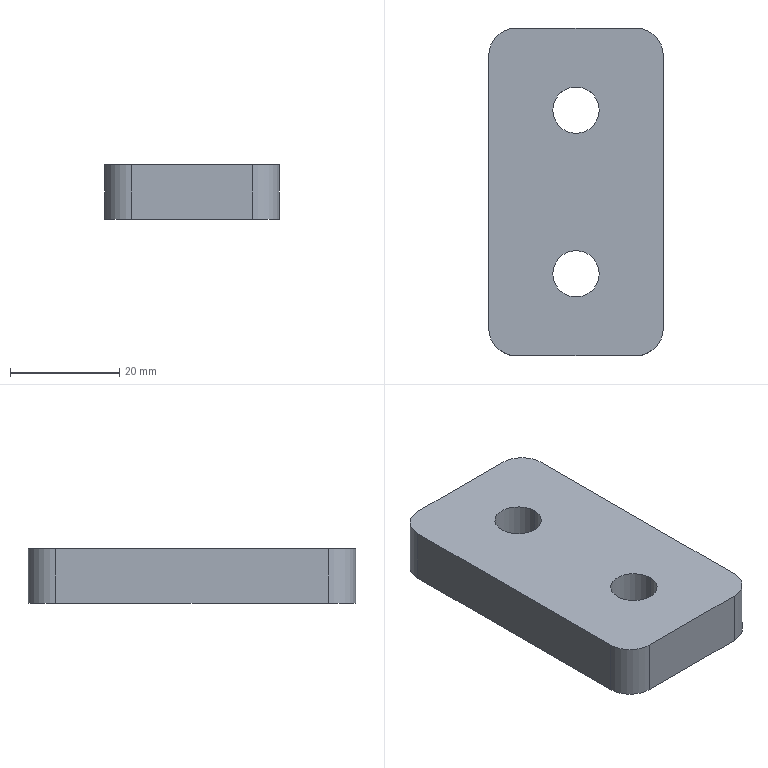Part | SolidWorks | features BaseBody 1 | 1 solid | 14 faces | box 32 x 60 x 10 mm | volume 17850 mm3 | cylinder 8 | plane 6 | commonest cylinder face diameters 8.5 x4 10 x4
STEP:
#1=CARTESIAN_POINT('',(-4.25,15.,0.));
#2=VERTEX_POINT('',#1);
#3=CARTESIAN_POINT('',(-4.25,15.,10.));
#4=VERTEX_POINT('',#3);
#5=CARTESIAN_POINT('',(-4.25,15.,-10.));
#6=DIRECTION('',(0.,0.,1.));
#7=VECTOR('',#6,1000.);
#8=LINE('',#5,#7);
#9=EDGE_CURVE('',#2,#4,#8,.T.);
#10=ORIENTED_EDGE('',*,*,#9,.F.);
#11=CARTESIAN_POINT('',(4.25,15.,0.));
#12=VERTEX_POINT('',#11);
#13=CARTESIAN_POINT('',(0.,15.,0.));
#14=DIRECTION('',(0.,0.,1.));
#15=DIRECTION('',(1.,0.,0.));
#16=AXIS2_PLACEMENT_3D('',#13,#14,#15);
#17=CIRCLE('',#16,4.25);
#18=EDGE_CURVE('',#12,#2,#17,.T.);
#19=ORIENTED_EDGE('',*,*,#18,.F.);
#20=CARTESIAN_POINT('',(4.25,15.,10.));
#21=VERTEX_POINT('',#20);
#22=CARTESIAN_POINT('',(4.25,15.,-10.));
#23=DIRECTION('',(0.,0.,1.));
#24=VECTOR('',#23,1000.);
#25=LINE('',#22,#24);
#26=EDGE_CURVE('',#12,#21,#25,.T.);
#27=ORIENTED_EDGE('',*,*,#26,.T.);
#28=CARTESIAN_POINT('',(0.,15.,10.));
#29=DIRECTION('',(0.,0.,1.));
#30=DIRECTION('',(1.,0.,0.));
#31=AXIS2_PLACEMENT_3D('',#28,#29,#30);
#32=CIRCLE('',#31,4.25);
#33=EDGE_CURVE('',#21,#4,#32,.T.);
#34=ORIENTED_EDGE('',*,*,#33,.T.);
#35=EDGE_LOOP('',(#10,#19,#27,#34));
#36=FACE_OUTER_BOUND('',#35,.T.);
#37=CARTESIAN_POINT('',(0.,15.,-10.));
#38=DIRECTION('',(0.,0.,1.));
#39=DIRECTION('',(1.,0.,0.));
#40=AXIS2_PLACEMENT_3D('',#37,#38,#39);
#41=CYLINDRICAL_SURFACE('',#40,4.25);
#42=ADVANCED_FACE('',(#36),#41,.F.);
#43=CARTESIAN_POINT('',(-4.25,-15.,0.));
#44=VERTEX_POINT('',#43);
#45=CARTESIAN_POINT('',(-4.25,-15.,10.));
#46=VERTEX_POINT('',#45);
#47=CARTESIAN_POINT('',(-4.25,-15.,-10.));
#48=DIRECTION('',(0.,0.,1.));
#49=VECTOR('',#48,1000.);
#50=LINE('',#47,#49);
#51=EDGE_CURVE('',#44,#46,#50,.T.);
#52=ORIENTED_EDGE('',*,*,#51,.F.);
#53=CARTESIAN_POINT('',(4.25,-15.,0.));
#54=VERTEX_POINT('',#53);
#55=CARTESIAN_POINT('',(0.,-15.,0.));
#56=DIRECTION('',(0.,0.,1.));
#57=DIRECTION('',(1.,0.,0.));
#58=AXIS2_PLACEMENT_3D('',#55,#56,#57);
#59=CIRCLE('',#58,4.25);
#60=EDGE_CURVE('',#54,#44,#59,.T.);
#61=ORIENTED_EDGE('',*,*,#60,.F.);
#62=CARTESIAN_POINT('',(4.25,-15.,10.));
#63=VERTEX_POINT('',#62);
#64=CARTESIAN_POINT('',(4.25,-15.,-10.));
#65=DIRECTION('',(0.,0.,1.));
#66=VECTOR('',#65,1000.);
#67=LINE('',#64,#66);
#68=EDGE_CURVE('',#54,#63,#67,.T.);
#69=ORIENTED_EDGE('',*,*,#68,.T.);
#70=CARTESIAN_POINT('',(0.,-15.,10.));
#71=DIRECTION('',(0.,0.,1.));
#72=DIRECTION('',(1.,0.,0.));
#73=AXIS2_PLACEMENT_3D('',#70,#71,#72);
#74=CIRCLE('',#73,4.25);
#75=EDGE_CURVE('',#63,#46,#74,.T.);
#76=ORIENTED_EDGE('',*,*,#75,.T.);
#77=EDGE_LOOP('',(#52,#61,#69,#76));
#78=FACE_OUTER_BOUND('',#77,.T.);
#79=CARTESIAN_POINT('',(0.,-15.,-10.));
#80=DIRECTION('',(0.,0.,1.));
#81=DIRECTION('',(1.,0.,0.));
#82=AXIS2_PLACEMENT_3D('',#79,#80,#81);
#83=CYLINDRICAL_SURFACE('',#82,4.25);
#84=ADVANCED_FACE('',(#78),#83,.F.);
#85=CARTESIAN_POINT('',(16.,25.,10.));
#86=VERTEX_POINT('',#85);
#87=CARTESIAN_POINT('',(11.,30.,10.));
#88=VERTEX_POINT('',#87);
#89=CARTESIAN_POINT('',(11.,25.,10.));
#90=DIRECTION('',(0.,0.,1.));
#91=DIRECTION('',(1.,0.,0.));
#92=AXIS2_PLACEMENT_3D('',#89,#90,#91);
#93=CIRCLE('',#92,5.);
#94=EDGE_CURVE('',#86,#88,#93,.T.);
#95=ORIENTED_EDGE('',*,*,#94,.F.);
#96=CARTESIAN_POINT('',(16.,25.,0.));
#97=VERTEX_POINT('',#96);
#98=CARTESIAN_POINT('',(16.,25.,10.));
#99=DIRECTION('',(0.,0.,1.));
#100=VECTOR('',#99,1000.);
#101=LINE('',#98,#100);
#102=EDGE_CURVE('',#97,#86,#101,.T.);
#103=ORIENTED_EDGE('',*,*,#102,.F.);
#104=CARTESIAN_POINT('',(11.,30.,0.));
#105=VERTEX_POINT('',#104);
#106=CARTESIAN_POINT('',(11.,25.,0.));
#107=DIRECTION('',(0.,0.,-1.));
#108=DIRECTION('',(1.,0.,0.));
#109=AXIS2_PLACEMENT_3D('',#106,#107,#108);
#110=CIRCLE('',#109,5.);
#111=EDGE_CURVE('',#105,#97,#110,.T.);
#112=ORIENTED_EDGE('',*,*,#111,.F.);
#113=CARTESIAN_POINT('',(11.,30.,10.));
#114=DIRECTION('',(0.,0.,-1.));
#115=VECTOR('',#114,1000.);
#116=LINE('',#113,#115);
#117=EDGE_CURVE('',#88,#105,#116,.T.);
#118=ORIENTED_EDGE('',*,*,#117,.F.);
#119=EDGE_LOOP('',(#95,#103,#112,#118));
#120=FACE_OUTER_BOUND('',#119,.T.);
#121=CARTESIAN_POINT('',(11.,25.,10.));
#122=DIRECTION('',(0.,0.,-1.));
#123=DIRECTION('',(-1.,0.,0.));
#124=AXIS2_PLACEMENT_3D('',#121,#122,#123);
#125=CYLINDRICAL_SURFACE('',#124,5.);
#126=ADVANCED_FACE('',(#120),#125,.T.);
#127=CARTESIAN_POINT('',(11.,-30.,10.));
#128=VERTEX_POINT('',#127);
#129=CARTESIAN_POINT('',(16.,-25.,10.));
#130=VERTEX_POINT('',#129);
#131=CARTESIAN_POINT('',(11.,-25.,10.));
#132=DIRECTION('',(0.,0.,1.));
#133=DIRECTION('',(1.,0.,0.));
#134=AXIS2_PLACEMENT_3D('',#131,#132,#133);
#135=CIRCLE('',#134,5.);
#136=EDGE_CURVE('',#128,#130,#135,.T.);
#137=ORIENTED_EDGE('',*,*,#136,.F.);
#138=CARTESIAN_POINT('',(11.,-30.,0.));
#139=VERTEX_POINT('',#138);
#140=CARTESIAN_POINT('',(11.,-30.,10.));
#141=DIRECTION('',(0.,0.,1.));
#142=VECTOR('',#141,1000.);
#143=LINE('',#140,#142);
#144=EDGE_CURVE('',#139,#128,#143,.T.);
#145=ORIENTED_EDGE('',*,*,#144,.F.);
#146=CARTESIAN_POINT('',(16.,-25.,0.));
#147=VERTEX_POINT('',#146);
#148=CARTESIAN_POINT('',(11.,-25.,0.));
#149=DIRECTION('',(0.,0.,-1.));
#150=DIRECTION('',(1.,0.,0.));
#151=AXIS2_PLACEMENT_3D('',#148,#149,#150);
#152=CIRCLE('',#151,5.);
#153=EDGE_CURVE('',#147,#139,#152,.T.);
#154=ORIENTED_EDGE('',*,*,#153,.F.);
#155=CARTESIAN_POINT('',(16.,-25.,10.));
#156=DIRECTION('',(0.,0.,-1.));
#157=VECTOR('',#156,1000.);
#158=LINE('',#155,#157);
#159=EDGE_CURVE('',#130,#147,#158,.T.);
#160=ORIENTED_EDGE('',*,*,#159,.F.);
#161=EDGE_LOOP('',(#137,#145,#154,#160));
#162=FACE_OUTER_BOUND('',#161,.T.);
#163=CARTESIAN_POINT('',(11.,-25.,10.));
#164=DIRECTION('',(0.,0.,-1.));
#165=DIRECTION('',(-1.,0.,0.));
#166=AXIS2_PLACEMENT_3D('',#163,#164,#165);
#167=CYLINDRICAL_SURFACE('',#166,5.);
#168=ADVANCED_FACE('',(#162),#167,.T.);
#169=CARTESIAN_POINT('',(-11.,30.,10.));
#170=VERTEX_POINT('',#169);
#171=CARTESIAN_POINT('',(-16.,25.,10.));
#172=VERTEX_POINT('',#171);
#173=CARTESIAN_POINT('',(-11.,25.,10.));
#174=DIRECTION('',(0.,0.,1.));
#175=DIRECTION('',(1.,0.,0.));
#176=AXIS2_PLACEMENT_3D('',#173,#174,#175);
#177=CIRCLE('',#176,5.);
#178=EDGE_CURVE('',#170,#172,#177,.T.);
#179=ORIENTED_EDGE('',*,*,#178,.F.);
#180=CARTESIAN_POINT('',(-11.,30.,0.));
#181=VERTEX_POINT('',#180);
#182=CARTESIAN_POINT('',(-11.,30.,10.));
#183=DIRECTION('',(0.,0.,1.));
#184=VECTOR('',#183,1000.);
#185=LINE('',#182,#184);
#186=EDGE_CURVE('',#181,#170,#185,.T.);
#187=ORIENTED_EDGE('',*,*,#186,.F.);
#188=CARTESIAN_POINT('',(-16.,25.,0.));
#189=VERTEX_POINT('',#188);
#190=CARTESIAN_POINT('',(-11.,25.,0.));
#191=DIRECTION('',(0.,0.,-1.));
#192=DIRECTION('',(1.,0.,0.));
#193=AXIS2_PLACEMENT_3D('',#190,#191,#192);
#194=CIRCLE('',#193,5.);
#195=EDGE_CURVE('',#189,#181,#194,.T.);
#196=ORIENTED_EDGE('',*,*,#195,.F.);
#197=CARTESIAN_POINT('',(-16.,25.,10.));
#198=DIRECTION('',(0.,0.,-1.));
#199=VECTOR('',#198,1000.);
#200=LINE('',#197,#199);
#201=EDGE_CURVE('',#172,#189,#200,.T.);
#202=ORIENTED_EDGE('',*,*,#201,.F.);
#203=EDGE_LOOP('',(#179,#187,#196,#202));
#204=FACE_OUTER_BOUND('',#203,.T.);
#205=CARTESIAN_POINT('',(-11.,25.,10.));
#206=DIRECTION('',(0.,0.,-1.));
#207=DIRECTION('',(-1.,0.,0.));
#208=AXIS2_PLACEMENT_3D('',#205,#206,#207);
#209=CYLINDRICAL_SURFACE('',#208,5.);
#210=ADVANCED_FACE('',(#204),#209,.T.);
#211=CARTESIAN_POINT('',(-16.,-25.,10.));
#212=VERTEX_POINT('',#211);
#213=CARTESIAN_POINT('',(-11.,-30.,10.));
#214=VERTEX_POINT('',#213);
#215=CARTESIAN_POINT('',(-11.,-25.,10.));
#216=DIRECTION('',(0.,0.,1.));
#217=DIRECTION('',(1.,0.,0.));
#218=AXIS2_PLACEMENT_3D('',#215,#216,#217);
#219=CIRCLE('',#218,5.);
#220=EDGE_CURVE('',#212,#214,#219,.T.);
#221=ORIENTED_EDGE('',*,*,#220,.F.);
#222=CARTESIAN_POINT('',(-16.,-25.,0.));
#223=VERTEX_POINT('',#222);
#224=CARTESIAN_POINT('',(-16.,-25.,10.));
#225=DIRECTION('',(0.,0.,1.));
#226=VECTOR('',#225,1000.);
#227=LINE('',#224,#226);
#228=EDGE_CURVE('',#223,#212,#227,.T.);
#229=ORIENTED_EDGE('',*,*,#228,.F.);
#230=CARTESIAN_POINT('',(-11.,-30.,0.));
#231=VERTEX_POINT('',#230);
#232=CARTESIAN_POINT('',(-11.,-25.,0.));
#233=DIRECTION('',(0.,0.,-1.));
#234=DIRECTION('',(1.,0.,0.));
#235=AXIS2_PLACEMENT_3D('',#232,#233,#234);
#236=CIRCLE('',#235,5.);
#237=EDGE_CURVE('',#231,#223,#236,.T.);
#238=ORIENTED_EDGE('',*,*,#237,.F.);
#239=CARTESIAN_POINT('',(-11.,-30.,10.));
#240=DIRECTION('',(0.,0.,-1.));
#241=VECTOR('',#240,1000.);
#242=LINE('',#239,#241);
#243=EDGE_CURVE('',#214,#231,#242,.T.);
#244=ORIENTED_EDGE('',*,*,#243,.F.);
#245=EDGE_LOOP('',(#221,#229,#238,#244));
#246=FACE_OUTER_BOUND('',#245,.T.);
#247=CARTESIAN_POINT('',(-11.,-25.,10.));
#248=DIRECTION('',(0.,0.,-1.));
#249=DIRECTION('',(-1.,0.,0.));
#250=AXIS2_PLACEMENT_3D('',#247,#248,#249);
#251=CYLINDRICAL_SURFACE('',#250,5.);
#252=ADVANCED_FACE('',(#246),#251,.T.);
#253=ORIENTED_EDGE('',*,*,#60,.T.);
#254=CARTESIAN_POINT('',(0.,-15.,0.));
#255=DIRECTION('',(0.,0.,1.));
#256=DIRECTION('',(1.,0.,0.));
#257=AXIS2_PLACEMENT_3D('',#254,#255,#256);
#258=CIRCLE('',#257,4.25);
#259=EDGE_CURVE('',#44,#54,#258,.T.);
#260=ORIENTED_EDGE('',*,*,#259,.T.);
#261=EDGE_LOOP('',(#253,#260));
#262=FACE_BOUND('',#261,.T.);
#263=ORIENTED_EDGE('',*,*,#18,.T.);
#264=CARTESIAN_POINT('',(0.,15.,0.));
#265=DIRECTION('',(0.,0.,1.));
#266=DIRECTION('',(1.,0.,0.));
#267=AXIS2_PLACEMENT_3D('',#264,#265,#266);
#268=CIRCLE('',#267,4.25);
#269=EDGE_CURVE('',#2,#12,#268,.T.);
#270=ORIENTED_EDGE('',*,*,#269,.T.);
#271=EDGE_LOOP('',(#263,#270));
#272=FACE_BOUND('',#271,.T.);
#273=CARTESIAN_POINT('',(-16.,-30.,0.));
#274=DIRECTION('',(1.,0.,0.));
#275=VECTOR('',#274,1000.);
#276=LINE('',#273,#275);
#277=EDGE_CURVE('',#231,#139,#276,.T.);
#278=ORIENTED_EDGE('',*,*,#277,.F.);
#279=ORIENTED_EDGE('',*,*,#237,.T.);
#280=CARTESIAN_POINT('',(-16.,30.,0.));
#281=DIRECTION('',(0.,-1.,0.));
#282=VECTOR('',#281,1000.);
#283=LINE('',#280,#282);
#284=EDGE_CURVE('',#189,#223,#283,.T.);
#285=ORIENTED_EDGE('',*,*,#284,.F.);
#286=ORIENTED_EDGE('',*,*,#195,.T.);
#287=CARTESIAN_POINT('',(-16.,30.,0.));
#288=DIRECTION('',(-1.,0.,0.));
#289=VECTOR('',#288,1000.);
#290=LINE('',#287,#289);
#291=EDGE_CURVE('',#105,#181,#290,.T.);
#292=ORIENTED_EDGE('',*,*,#291,.F.);
#293=ORIENTED_EDGE('',*,*,#111,.T.);
#294=CARTESIAN_POINT('',(16.,30.,0.));
#295=DIRECTION('',(0.,1.,0.));
#296=VECTOR('',#295,1000.);
#297=LINE('',#294,#296);
#298=EDGE_CURVE('',#147,#97,#297,.T.);
#299=ORIENTED_EDGE('',*,*,#298,.F.);
#300=ORIENTED_EDGE('',*,*,#153,.T.);
#301=EDGE_LOOP('',(#278,#279,#285,#286,#292,#293,#299,#300));
#302=FACE_OUTER_BOUND('',#301,.T.);
#303=CARTESIAN_POINT('',(0.,0.,0.));
#304=DIRECTION('',(0.,0.,1.));
#305=DIRECTION('',(1.,0.,0.));
#306=AXIS2_PLACEMENT_3D('',#303,#304,#305);
#307=PLANE('',#306);
#308=ADVANCED_FACE('',(#262,#272,#302),#307,.F.);
#309=ORIENTED_EDGE('',*,*,#75,.F.);
#310=CARTESIAN_POINT('',(0.,-15.,10.));
#311=DIRECTION('',(0.,0.,1.));
#312=DIRECTION('',(1.,0.,0.));
#313=AXIS2_PLACEMENT_3D('',#310,#311,#312);
#314=CIRCLE('',#313,4.25);
#315=EDGE_CURVE('',#46,#63,#314,.T.);
#316=ORIENTED_EDGE('',*,*,#315,.F.);
#317=EDGE_LOOP('',(#309,#316));
#318=FACE_BOUND('',#317,.T.);
#319=ORIENTED_EDGE('',*,*,#33,.F.);
#320=CARTESIAN_POINT('',(0.,15.,10.));
#321=DIRECTION('',(0.,0.,1.));
#322=DIRECTION('',(1.,0.,0.));
#323=AXIS2_PLACEMENT_3D('',#320,#321,#322);
#324=CIRCLE('',#323,4.25);
#325=EDGE_CURVE('',#4,#21,#324,.T.);
#326=ORIENTED_EDGE('',*,*,#325,.F.);
#327=EDGE_LOOP('',(#319,#326));
#328=FACE_BOUND('',#327,.T.);
#329=CARTESIAN_POINT('',(-16.,30.,10.));
#330=DIRECTION('',(0.,-1.,0.));
#331=VECTOR('',#330,1000.);
#332=LINE('',#329,#331);
#333=EDGE_CURVE('',#172,#212,#332,.T.);
#334=ORIENTED_EDGE('',*,*,#333,.T.);
#335=ORIENTED_EDGE('',*,*,#220,.T.);
#336=CARTESIAN_POINT('',(-16.,-30.,10.));
#337=DIRECTION('',(1.,0.,0.));
#338=VECTOR('',#337,1000.);
#339=LINE('',#336,#338);
#340=EDGE_CURVE('',#214,#128,#339,.T.);
#341=ORIENTED_EDGE('',*,*,#340,.T.);
#342=ORIENTED_EDGE('',*,*,#136,.T.);
#343=CARTESIAN_POINT('',(16.,30.,10.));
#344=DIRECTION('',(0.,1.,0.));
#345=VECTOR('',#344,1000.);
#346=LINE('',#343,#345);
#347=EDGE_CURVE('',#130,#86,#346,.T.);
#348=ORIENTED_EDGE('',*,*,#347,.T.);
#349=ORIENTED_EDGE('',*,*,#94,.T.);
#350=CARTESIAN_POINT('',(-16.,30.,10.));
#351=DIRECTION('',(-1.,0.,0.));
#352=VECTOR('',#351,1000.);
#353=LINE('',#350,#352);
#354=EDGE_CURVE('',#88,#170,#353,.T.);
#355=ORIENTED_EDGE('',*,*,#354,.T.);
#356=ORIENTED_EDGE('',*,*,#178,.T.);
#357=EDGE_LOOP('',(#334,#335,#341,#342,#348,#349,#355,#356));
#358=FACE_OUTER_BOUND('',#357,.T.);
#359=CARTESIAN_POINT('',(0.,0.,10.));
#360=DIRECTION('',(0.,0.,1.));
#361=DIRECTION('',(1.,0.,0.));
#362=AXIS2_PLACEMENT_3D('',#359,#360,#361);
#363=PLANE('',#362);
#364=ADVANCED_FACE('',(#318,#328,#358),#363,.T.);
#365=ORIENTED_EDGE('',*,*,#340,.F.);
#366=ORIENTED_EDGE('',*,*,#243,.T.);
#367=ORIENTED_EDGE('',*,*,#277,.T.);
#368=ORIENTED_EDGE('',*,*,#144,.T.);
#369=EDGE_LOOP('',(#365,#366,#367,#368));
#370=FACE_OUTER_BOUND('',#369,.T.);
#371=CARTESIAN_POINT('',(-16.,-30.,10.));
#372=DIRECTION('',(0.,1.,0.));
#373=DIRECTION('',(1.,0.,0.));
#374=AXIS2_PLACEMENT_3D('',#371,#372,#373);
#375=PLANE('',#374);
#376=ADVANCED_FACE('',(#370),#375,.F.);
#377=ORIENTED_EDGE('',*,*,#284,.T.);
#378=ORIENTED_EDGE('',*,*,#228,.T.);
#379=ORIENTED_EDGE('',*,*,#333,.F.);
#380=ORIENTED_EDGE('',*,*,#201,.T.);
#381=EDGE_LOOP('',(#377,#378,#379,#380));
#382=FACE_OUTER_BOUND('',#381,.T.);
#383=CARTESIAN_POINT('',(-16.,30.,10.));
#384=DIRECTION('',(1.,0.,0.));
#385=DIRECTION('',(0.,1.,0.));
#386=AXIS2_PLACEMENT_3D('',#383,#384,#385);
#387=PLANE('',#386);
#388=ADVANCED_FACE('',(#382),#387,.F.);
#389=ORIENTED_EDGE('',*,*,#291,.T.);
#390=ORIENTED_EDGE('',*,*,#186,.T.);
#391=ORIENTED_EDGE('',*,*,#354,.F.);
#392=ORIENTED_EDGE('',*,*,#117,.T.);
#393=EDGE_LOOP('',(#389,#390,#391,#392));
#394=FACE_OUTER_BOUND('',#393,.T.);
#395=CARTESIAN_POINT('',(-16.,30.,10.));
#396=DIRECTION('',(0.,-1.,0.));
#397=DIRECTION('',(0.,0.,-1.));
#398=AXIS2_PLACEMENT_3D('',#395,#396,#397);
#399=PLANE('',#398);
#400=ADVANCED_FACE('',(#394),#399,.F.);
#401=ORIENTED_EDGE('',*,*,#347,.F.);
#402=ORIENTED_EDGE('',*,*,#159,.T.);
#403=ORIENTED_EDGE('',*,*,#298,.T.);
#404=ORIENTED_EDGE('',*,*,#102,.T.);
#405=EDGE_LOOP('',(#401,#402,#403,#404));
#406=FACE_OUTER_BOUND('',#405,.T.);
#407=CARTESIAN_POINT('',(16.,30.,10.));
#408=DIRECTION('',(-1.,0.,0.));
#409=DIRECTION('',(0.,1.,0.));
#410=AXIS2_PLACEMENT_3D('',#407,#408,#409);
#411=PLANE('',#410);
#412=ADVANCED_FACE('',(#406),#411,.F.);
#413=ORIENTED_EDGE('',*,*,#259,.F.);
#414=ORIENTED_EDGE('',*,*,#51,.T.);
#415=ORIENTED_EDGE('',*,*,#315,.T.);
#416=ORIENTED_EDGE('',*,*,#68,.F.);
#417=EDGE_LOOP('',(#413,#414,#415,#416));
#418=FACE_OUTER_BOUND('',#417,.T.);
#419=CARTESIAN_POINT('',(0.,-15.,-10.));
#420=DIRECTION('',(0.,0.,1.));
#421=DIRECTION('',(1.,0.,0.));
#422=AXIS2_PLACEMENT_3D('',#419,#420,#421);
#423=CYLINDRICAL_SURFACE('',#422,4.25);
#424=ADVANCED_FACE('',(#418),#423,.F.);
#425=ORIENTED_EDGE('',*,*,#269,.F.);
#426=ORIENTED_EDGE('',*,*,#9,.T.);
#427=ORIENTED_EDGE('',*,*,#325,.T.);
#428=ORIENTED_EDGE('',*,*,#26,.F.);
#429=EDGE_LOOP('',(#425,#426,#427,#428));
#430=FACE_OUTER_BOUND('',#429,.T.);
#431=CARTESIAN_POINT('',(0.,15.,-10.));
#432=DIRECTION('',(0.,0.,1.));
#433=DIRECTION('',(1.,0.,0.));
#434=AXIS2_PLACEMENT_3D('',#431,#432,#433);
#435=CYLINDRICAL_SURFACE('',#434,4.25);
#436=ADVANCED_FACE('',(#430),#435,.F.);
#437=CLOSED_SHELL('',(#42,#84,#126,#168,#210,#252,#308,#364,#376,#388,#400,#412,#424,#436));
#438=MANIFOLD_SOLID_BREP('',#437);
#439=CARTESIAN_POINT('',(0.,0.,0.));
#440=DIRECTION('',(0.,0.,1.));
#441=DIRECTION('',(1.,0.,0.));
#442=AXIS2_PLACEMENT_3D('',#439,#440,#441);
#443=(LENGTH_UNIT()NAMED_UNIT(*)SI_UNIT(.MILLI.,.METRE.));
#444=UNCERTAINTY_MEASURE_WITH_UNIT(LENGTH_MEASURE(0.00001),#443,'','');
#445=(NAMED_UNIT(*)PLANE_ANGLE_UNIT()SI_UNIT($,.RADIAN.));
#446=(NAMED_UNIT(*)SI_UNIT($,.STERADIAN.)SOLID_ANGLE_UNIT());
#447=(GEOMETRIC_REPRESENTATION_CONTEXT(3)GLOBAL_UNCERTAINTY_ASSIGNED_CONTEXT((#444))GLOBAL_UNIT_ASSIGNED_CONTEXT((#443,#445,#446))REPRESENTATION_CONTEXT('',''));
#448=ADVANCED_BREP_SHAPE_REPRESENTATION('',(#438,#442),#447);